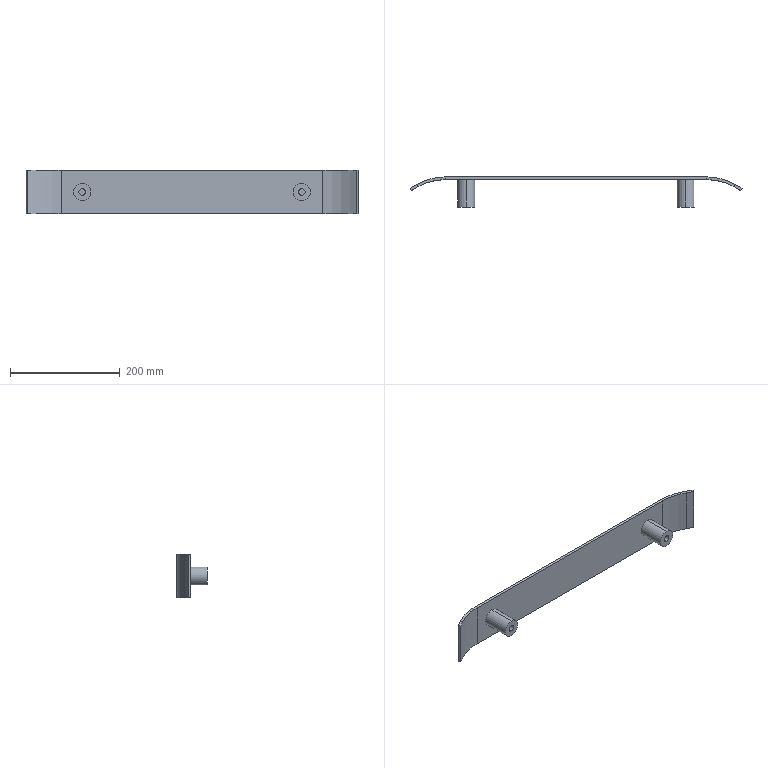Part | SolidWorks | features ICE 2, FlatPattern 1, SMBaseFlange 1, SheetMetal 1 | 1 solid | 34 faces | box 604.961 x 55 x 80 mm | volume 316837 mm3 | plane 22 | cylinder 12 | commonest cylinder face diameters 12 x4 32 x4 200 x2 210 x2
STEP:
#1=CARTESIAN_POINT('',(200.,-15.,6.));
#2=VERTEX_POINT('',#1);
#3=CARTESIAN_POINT('',(200.,-15.,-6.));
#4=VERTEX_POINT('',#3);
#5=CARTESIAN_POINT('',(200.,-15.,0.));
#6=DIRECTION('',(0.,-1.,0.));
#7=DIRECTION('',(0.,0.,-1.));
#8=AXIS2_PLACEMENT_3D('',#5,#6,#7);
#9=CIRCLE('',#8,6.);
#10=EDGE_CURVE('',#2,#4,#9,.T.);
#11=ORIENTED_EDGE('',*,*,#10,.F.);
#12=CARTESIAN_POINT('',(200.,-50.,6.));
#13=VERTEX_POINT('',#12);
#14=CARTESIAN_POINT('',(200.,-15.,6.));
#15=DIRECTION('',(0.,-1.,0.));
#16=VECTOR('',#15,1000.);
#17=LINE('',#14,#16);
#18=EDGE_CURVE('',#2,#13,#17,.T.);
#19=ORIENTED_EDGE('',*,*,#18,.T.);
#20=CARTESIAN_POINT('',(200.,-50.,-6.));
#21=VERTEX_POINT('',#20);
#22=CARTESIAN_POINT('',(200.,-50.,0.));
#23=DIRECTION('',(0.,-1.,0.));
#24=DIRECTION('',(0.,0.,-1.));
#25=AXIS2_PLACEMENT_3D('',#22,#23,#24);
#26=CIRCLE('',#25,6.);
#27=EDGE_CURVE('',#13,#21,#26,.T.);
#28=ORIENTED_EDGE('',*,*,#27,.T.);
#29=CARTESIAN_POINT('',(200.,-15.,-6.));
#30=DIRECTION('',(0.,-1.,0.));
#31=VECTOR('',#30,1000.);
#32=LINE('',#29,#31);
#33=EDGE_CURVE('',#4,#21,#32,.T.);
#34=ORIENTED_EDGE('',*,*,#33,.F.);
#35=EDGE_LOOP('',(#11,#19,#28,#34));
#36=FACE_OUTER_BOUND('',#35,.T.);
#37=CARTESIAN_POINT('',(200.,-15.,0.));
#38=DIRECTION('',(0.,-1.,0.));
#39=DIRECTION('',(0.,0.,-1.));
#40=AXIS2_PLACEMENT_3D('',#37,#38,#39);
#41=CYLINDRICAL_SURFACE('',#40,6.);
#42=ADVANCED_FACE('',(#36),#41,.F.);
#43=CARTESIAN_POINT('',(-200.,-15.,6.));
#44=VERTEX_POINT('',#43);
#45=CARTESIAN_POINT('',(-200.,-15.,-6.));
#46=VERTEX_POINT('',#45);
#47=CARTESIAN_POINT('',(-200.,-15.,0.));
#48=DIRECTION('',(0.,-1.,0.));
#49=DIRECTION('',(0.,0.,-1.));
#50=AXIS2_PLACEMENT_3D('',#47,#48,#49);
#51=CIRCLE('',#50,6.);
#52=EDGE_CURVE('',#44,#46,#51,.T.);
#53=ORIENTED_EDGE('',*,*,#52,.F.);
#54=CARTESIAN_POINT('',(-200.,-50.,6.));
#55=VERTEX_POINT('',#54);
#56=CARTESIAN_POINT('',(-200.,-15.,6.));
#57=DIRECTION('',(0.,-1.,0.));
#58=VECTOR('',#57,1000.);
#59=LINE('',#56,#58);
#60=EDGE_CURVE('',#44,#55,#59,.T.);
#61=ORIENTED_EDGE('',*,*,#60,.T.);
#62=CARTESIAN_POINT('',(-200.,-50.,-6.));
#63=VERTEX_POINT('',#62);
#64=CARTESIAN_POINT('',(-200.,-50.,0.));
#65=DIRECTION('',(0.,-1.,0.));
#66=DIRECTION('',(0.,0.,-1.));
#67=AXIS2_PLACEMENT_3D('',#64,#65,#66);
#68=CIRCLE('',#67,6.);
#69=EDGE_CURVE('',#55,#63,#68,.T.);
#70=ORIENTED_EDGE('',*,*,#69,.T.);
#71=CARTESIAN_POINT('',(-200.,-15.,-6.));
#72=DIRECTION('',(0.,-1.,0.));
#73=VECTOR('',#72,1000.);
#74=LINE('',#71,#73);
#75=EDGE_CURVE('',#46,#63,#74,.T.);
#76=ORIENTED_EDGE('',*,*,#75,.F.);
#77=EDGE_LOOP('',(#53,#61,#70,#76));
#78=FACE_OUTER_BOUND('',#77,.T.);
#79=CARTESIAN_POINT('',(-200.,-15.,0.));
#80=DIRECTION('',(0.,-1.,0.));
#81=DIRECTION('',(0.,0.,-1.));
#82=AXIS2_PLACEMENT_3D('',#79,#80,#81);
#83=CYLINDRICAL_SURFACE('',#82,6.);
#84=ADVANCED_FACE('',(#78),#83,.F.);
#85=CARTESIAN_POINT('',(-200.,-50.,-16.));
#86=VERTEX_POINT('',#85);
#87=CARTESIAN_POINT('',(-200.,-50.,16.));
#88=VERTEX_POINT('',#87);
#89=CARTESIAN_POINT('',(-200.,-50.,0.));
#90=DIRECTION('',(0.,-1.,0.));
#91=DIRECTION('',(0.,0.,-1.));
#92=AXIS2_PLACEMENT_3D('',#89,#90,#91);
#93=CIRCLE('',#92,16.);
#94=EDGE_CURVE('',#86,#88,#93,.T.);
#95=ORIENTED_EDGE('',*,*,#94,.F.);
#96=CARTESIAN_POINT('',(-200.,0.,-16.));
#97=VERTEX_POINT('',#96);
#98=CARTESIAN_POINT('',(-200.,-50.,-16.));
#99=DIRECTION('',(0.,1.,0.));
#100=VECTOR('',#99,1000.);
#101=LINE('',#98,#100);
#102=EDGE_CURVE('',#86,#97,#101,.T.);
#103=ORIENTED_EDGE('',*,*,#102,.T.);
#104=CARTESIAN_POINT('',(-200.,0.,16.));
#105=VERTEX_POINT('',#104);
#106=CARTESIAN_POINT('',(-200.,0.,0.));
#107=DIRECTION('',(0.,-1.,0.));
#108=DIRECTION('',(0.,0.,-1.));
#109=AXIS2_PLACEMENT_3D('',#106,#107,#108);
#110=CIRCLE('',#109,16.);
#111=EDGE_CURVE('',#97,#105,#110,.T.);
#112=ORIENTED_EDGE('',*,*,#111,.T.);
#113=CARTESIAN_POINT('',(-200.,-50.,16.));
#114=DIRECTION('',(0.,1.,0.));
#115=VECTOR('',#114,1000.);
#116=LINE('',#113,#115);
#117=EDGE_CURVE('',#88,#105,#116,.T.);
#118=ORIENTED_EDGE('',*,*,#117,.F.);
#119=EDGE_LOOP('',(#95,#103,#112,#118));
#120=FACE_OUTER_BOUND('',#119,.T.);
#121=CARTESIAN_POINT('',(-200.,-50.,0.));
#122=DIRECTION('',(0.,1.,0.));
#123=DIRECTION('',(0.,0.,1.));
#124=AXIS2_PLACEMENT_3D('',#121,#122,#123);
#125=CYLINDRICAL_SURFACE('',#124,16.);
#126=ADVANCED_FACE('',(#120),#125,.T.);
#127=CARTESIAN_POINT('',(200.,-50.,-16.));
#128=VERTEX_POINT('',#127);
#129=CARTESIAN_POINT('',(200.,-50.,16.));
#130=VERTEX_POINT('',#129);
#131=CARTESIAN_POINT('',(200.,-50.,0.));
#132=DIRECTION('',(0.,-1.,0.));
#133=DIRECTION('',(0.,0.,-1.));
#134=AXIS2_PLACEMENT_3D('',#131,#132,#133);
#135=CIRCLE('',#134,16.);
#136=EDGE_CURVE('',#128,#130,#135,.T.);
#137=ORIENTED_EDGE('',*,*,#136,.F.);
#138=CARTESIAN_POINT('',(200.,0.,-16.));
#139=VERTEX_POINT('',#138);
#140=CARTESIAN_POINT('',(200.,-50.,-16.));
#141=DIRECTION('',(0.,1.,0.));
#142=VECTOR('',#141,1000.);
#143=LINE('',#140,#142);
#144=EDGE_CURVE('',#128,#139,#143,.T.);
#145=ORIENTED_EDGE('',*,*,#144,.T.);
#146=CARTESIAN_POINT('',(200.,0.,16.));
#147=VERTEX_POINT('',#146);
#148=CARTESIAN_POINT('',(200.,0.,0.));
#149=DIRECTION('',(0.,-1.,0.));
#150=DIRECTION('',(0.,0.,-1.));
#151=AXIS2_PLACEMENT_3D('',#148,#149,#150);
#152=CIRCLE('',#151,16.);
#153=EDGE_CURVE('',#139,#147,#152,.T.);
#154=ORIENTED_EDGE('',*,*,#153,.T.);
#155=CARTESIAN_POINT('',(200.,-50.,16.));
#156=DIRECTION('',(0.,1.,0.));
#157=VECTOR('',#156,1000.);
#158=LINE('',#155,#157);
#159=EDGE_CURVE('',#130,#147,#158,.T.);
#160=ORIENTED_EDGE('',*,*,#159,.F.);
#161=EDGE_LOOP('',(#137,#145,#154,#160));
#162=FACE_OUTER_BOUND('',#161,.T.);
#163=CARTESIAN_POINT('',(200.,-50.,0.));
#164=DIRECTION('',(0.,1.,0.));
#165=DIRECTION('',(0.,0.,1.));
#166=AXIS2_PLACEMENT_3D('',#163,#164,#165);
#167=CYLINDRICAL_SURFACE('',#166,16.);
#168=ADVANCED_FACE('',(#162),#167,.T.);
#169=CARTESIAN_POINT('',(238.444,0.,40.));
#170=VERTEX_POINT('',#169);
#171=CARTESIAN_POINT('',(238.444,5.,40.));
#172=VERTEX_POINT('',#171);
#173=CARTESIAN_POINT('',(238.444,0.,40.));
#174=DIRECTION('',(0.,1.,0.));
#175=VECTOR('',#174,1000.);
#176=LINE('',#173,#175);
#177=EDGE_CURVE('',#170,#172,#176,.T.);
#178=ORIENTED_EDGE('',*,*,#177,.F.);
#179=CARTESIAN_POINT('',(288.057,-13.176,40.));
#180=VERTEX_POINT('',#179);
#181=CARTESIAN_POINT('',(238.444,-100.,40.));
#182=DIRECTION('',(0.,0.,1.));
#183=DIRECTION('',(-1.,0.,0.));
#184=AXIS2_PLACEMENT_3D('',#181,#182,#183);
#185=CIRCLE('',#184,100.);
#186=EDGE_CURVE('',#180,#170,#185,.T.);
#187=ORIENTED_EDGE('',*,*,#186,.F.);
#188=CARTESIAN_POINT('',(290.538,-8.834,40.));
#189=VERTEX_POINT('',#188);
#190=CARTESIAN_POINT('',(290.538,-8.834,40.));
#191=DIRECTION('',(-0.4961,-0.8682,0.));
#192=VECTOR('',#191,1000.);
#193=LINE('',#190,#192);
#194=EDGE_CURVE('',#189,#180,#193,.T.);
#195=ORIENTED_EDGE('',*,*,#194,.F.);
#196=CARTESIAN_POINT('',(238.444,-100.,40.));
#197=DIRECTION('',(0.,0.,1.));
#198=DIRECTION('',(1.,0.,0.));
#199=AXIS2_PLACEMENT_3D('',#196,#197,#198);
#200=CIRCLE('',#199,105.);
#201=EDGE_CURVE('',#189,#172,#200,.T.);
#202=ORIENTED_EDGE('',*,*,#201,.T.);
#203=EDGE_LOOP('',(#178,#187,#195,#202));
#204=FACE_OUTER_BOUND('',#203,.T.);
#205=CARTESIAN_POINT('',(238.444,0.,40.));
#206=DIRECTION('',(0.,0.,1.));
#207=DIRECTION('',(1.,0.,0.));
#208=AXIS2_PLACEMENT_3D('',#205,#206,#207);
#209=PLANE('',#208);
#210=ADVANCED_FACE('',(#204),#209,.T.);
#211=CARTESIAN_POINT('',(-238.444,0.,40.));
#212=VERTEX_POINT('',#211);
#213=CARTESIAN_POINT('',(-265.,0.,40.));
#214=DIRECTION('',(-1.,0.,0.));
#215=VECTOR('',#214,1000.);
#216=LINE('',#213,#215);
#217=EDGE_CURVE('',#170,#212,#216,.T.);
#218=ORIENTED_EDGE('',*,*,#217,.F.);
#219=ORIENTED_EDGE('',*,*,#177,.T.);
#220=CARTESIAN_POINT('',(-238.444,5.,40.));
#221=VERTEX_POINT('',#220);
#222=CARTESIAN_POINT('',(-265.,5.,40.));
#223=DIRECTION('',(-1.,0.,0.));
#224=VECTOR('',#223,1000.);
#225=LINE('',#222,#224);
#226=EDGE_CURVE('',#172,#221,#225,.T.);
#227=ORIENTED_EDGE('',*,*,#226,.T.);
#228=CARTESIAN_POINT('',(-238.444,5.,40.));
#229=DIRECTION('',(0.,-1.,0.));
#230=VECTOR('',#229,1000.);
#231=LINE('',#228,#230);
#232=EDGE_CURVE('',#221,#212,#231,.T.);
#233=ORIENTED_EDGE('',*,*,#232,.T.);
#234=EDGE_LOOP('',(#218,#219,#227,#233));
#235=FACE_OUTER_BOUND('',#234,.T.);
#236=CARTESIAN_POINT('',(290.538,-8.834,40.));
#237=DIRECTION('',(0.,0.,1.));
#238=DIRECTION('',(1.,0.,0.));
#239=AXIS2_PLACEMENT_3D('',#236,#237,#238);
#240=PLANE('',#239);
#241=ADVANCED_FACE('',(#235),#240,.T.);
#242=CARTESIAN_POINT('',(288.057,-13.176,-40.));
#243=VERTEX_POINT('',#242);
#244=CARTESIAN_POINT('',(290.538,-8.834,-40.));
#245=VERTEX_POINT('',#244);
#246=CARTESIAN_POINT('',(288.057,-13.176,-40.));
#247=DIRECTION('',(0.4961,0.8682,0.));
#248=VECTOR('',#247,1000.);
#249=LINE('',#246,#248);
#250=EDGE_CURVE('',#243,#245,#249,.T.);
#251=ORIENTED_EDGE('',*,*,#250,.F.);
#252=CARTESIAN_POINT('',(238.444,0.,-40.));
#253=VERTEX_POINT('',#252);
#254=CARTESIAN_POINT('',(238.444,-100.,-40.));
#255=DIRECTION('',(0.,0.,1.));
#256=DIRECTION('',(-1.,0.,0.));
#257=AXIS2_PLACEMENT_3D('',#254,#255,#256);
#258=CIRCLE('',#257,100.);
#259=EDGE_CURVE('',#243,#253,#258,.T.);
#260=ORIENTED_EDGE('',*,*,#259,.T.);
#261=CARTESIAN_POINT('',(238.444,5.,-40.));
#262=VERTEX_POINT('',#261);
#263=CARTESIAN_POINT('',(238.444,5.,-40.));
#264=DIRECTION('',(0.,-1.,0.));
#265=VECTOR('',#264,1000.);
#266=LINE('',#263,#265);
#267=EDGE_CURVE('',#262,#253,#266,.T.);
#268=ORIENTED_EDGE('',*,*,#267,.F.);
#269=CARTESIAN_POINT('',(238.444,-100.,-40.));
#270=DIRECTION('',(0.,0.,1.));
#271=DIRECTION('',(1.,0.,0.));
#272=AXIS2_PLACEMENT_3D('',#269,#270,#271);
#273=CIRCLE('',#272,105.);
#274=EDGE_CURVE('',#245,#262,#273,.T.);
#275=ORIENTED_EDGE('',*,*,#274,.F.);
#276=EDGE_LOOP('',(#251,#260,#268,#275));
#277=FACE_OUTER_BOUND('',#276,.T.);
#278=CARTESIAN_POINT('',(288.057,-13.176,-40.));
#279=DIRECTION('',(0.,0.,-1.));
#280=DIRECTION('',(-1.,0.,0.));
#281=AXIS2_PLACEMENT_3D('',#278,#279,#280);
#282=PLANE('',#281);
#283=ADVANCED_FACE('',(#277),#282,.T.);
#284=CARTESIAN_POINT('',(300.,-20.,-40.));
#285=VERTEX_POINT('',#284);
#286=CARTESIAN_POINT('',(265.,0.,-40.));
#287=DIRECTION('',(-0.8682,0.4961,0.));
#288=VECTOR('',#287,1000.);
#289=LINE('',#286,#288);
#290=EDGE_CURVE('',#285,#243,#289,.T.);
#291=ORIENTED_EDGE('',*,*,#290,.T.);
#292=ORIENTED_EDGE('',*,*,#250,.T.);
#293=CARTESIAN_POINT('',(302.481,-15.659,-40.));
#294=VERTEX_POINT('',#293);
#295=CARTESIAN_POINT('',(267.481,4.341,-40.));
#296=DIRECTION('',(-0.8682,0.4961,0.));
#297=VECTOR('',#296,1000.);
#298=LINE('',#295,#297);
#299=EDGE_CURVE('',#294,#245,#298,.T.);
#300=ORIENTED_EDGE('',*,*,#299,.F.);
#301=CARTESIAN_POINT('',(302.481,-15.659,-40.));
#302=DIRECTION('',(-0.4961,-0.8682,0.));
#303=VECTOR('',#302,1000.);
#304=LINE('',#301,#303);
#305=EDGE_CURVE('',#294,#285,#304,.T.);
#306=ORIENTED_EDGE('',*,*,#305,.T.);
#307=EDGE_LOOP('',(#291,#292,#300,#306));
#308=FACE_OUTER_BOUND('',#307,.T.);
#309=CARTESIAN_POINT('',(238.444,5.,-40.));
#310=DIRECTION('',(0.,0.,-1.));
#311=DIRECTION('',(-1.,0.,0.));
#312=AXIS2_PLACEMENT_3D('',#309,#310,#311);
#313=PLANE('',#312);
#314=ADVANCED_FACE('',(#308),#313,.T.);
#315=CARTESIAN_POINT('',(-288.057,-13.176,40.));
#316=VERTEX_POINT('',#315);
#317=CARTESIAN_POINT('',(-290.538,-8.834,40.));
#318=VERTEX_POINT('',#317);
#319=CARTESIAN_POINT('',(-288.057,-13.176,40.));
#320=DIRECTION('',(-0.4961,0.8682,0.));
#321=VECTOR('',#320,1000.);
#322=LINE('',#319,#321);
#323=EDGE_CURVE('',#316,#318,#322,.T.);
#324=ORIENTED_EDGE('',*,*,#323,.F.);
#325=CARTESIAN_POINT('',(-238.444,-100.,40.));
#326=DIRECTION('',(0.,0.,1.));
#327=DIRECTION('',(-1.,0.,0.));
#328=AXIS2_PLACEMENT_3D('',#325,#326,#327);
#329=CIRCLE('',#328,100.);
#330=EDGE_CURVE('',#212,#316,#329,.T.);
#331=ORIENTED_EDGE('',*,*,#330,.F.);
#332=ORIENTED_EDGE('',*,*,#232,.F.);
#333=CARTESIAN_POINT('',(-238.444,-100.,40.));
#334=DIRECTION('',(0.,0.,1.));
#335=DIRECTION('',(1.,0.,0.));
#336=AXIS2_PLACEMENT_3D('',#333,#334,#335);
#337=CIRCLE('',#336,105.);
#338=EDGE_CURVE('',#221,#318,#337,.T.);
#339=ORIENTED_EDGE('',*,*,#338,.T.);
#340=EDGE_LOOP('',(#324,#331,#332,#339));
#341=FACE_OUTER_BOUND('',#340,.T.);
#342=CARTESIAN_POINT('',(-288.057,-13.176,40.));
#343=DIRECTION('',(0.,0.,1.));
#344=DIRECTION('',(1.,0.,0.));
#345=AXIS2_PLACEMENT_3D('',#342,#343,#344);
#346=PLANE('',#345);
#347=ADVANCED_FACE('',(#341),#346,.T.);
#348=CARTESIAN_POINT('',(-300.,-20.,40.));
#349=VERTEX_POINT('',#348);
#350=CARTESIAN_POINT('',(-265.,0.,40.));
#351=DIRECTION('',(-0.8682,-0.4961,0.));
#352=VECTOR('',#351,1000.);
#353=LINE('',#350,#352);
#354=EDGE_CURVE('',#316,#349,#353,.T.);
#355=ORIENTED_EDGE('',*,*,#354,.F.);
#356=ORIENTED_EDGE('',*,*,#323,.T.);
#357=CARTESIAN_POINT('',(-302.481,-15.659,40.));
#358=VERTEX_POINT('',#357);
#359=CARTESIAN_POINT('',(-267.481,4.341,40.));
#360=DIRECTION('',(-0.8682,-0.4961,0.));
#361=VECTOR('',#360,1000.);
#362=LINE('',#359,#361);
#363=EDGE_CURVE('',#318,#358,#362,.T.);
#364=ORIENTED_EDGE('',*,*,#363,.T.);
#365=CARTESIAN_POINT('',(-300.,-20.,40.));
#366=DIRECTION('',(-0.4961,0.8682,0.));
#367=VECTOR('',#366,1000.);
#368=LINE('',#365,#367);
#369=EDGE_CURVE('',#349,#358,#368,.T.);
#370=ORIENTED_EDGE('',*,*,#369,.F.);
#371=EDGE_LOOP('',(#355,#356,#364,#370));
#372=FACE_OUTER_BOUND('',#371,.T.);
#373=CARTESIAN_POINT('',(-238.444,5.,40.));
#374=DIRECTION('',(0.,0.,1.));
#375=DIRECTION('',(1.,0.,0.));
#376=AXIS2_PLACEMENT_3D('',#373,#374,#375);
#377=PLANE('',#376);
#378=ADVANCED_FACE('',(#372),#377,.T.);
#379=CARTESIAN_POINT('',(-238.444,0.,-40.));
#380=VERTEX_POINT('',#379);
#381=CARTESIAN_POINT('',(-238.444,5.,-40.));
#382=VERTEX_POINT('',#381);
#383=CARTESIAN_POINT('',(-238.444,0.,-40.));
#384=DIRECTION('',(0.,1.,0.));
#385=VECTOR('',#384,1000.);
#386=LINE('',#383,#385);
#387=EDGE_CURVE('',#380,#382,#386,.T.);
#388=ORIENTED_EDGE('',*,*,#387,.F.);
#389=CARTESIAN_POINT('',(-288.057,-13.176,-40.));
#390=VERTEX_POINT('',#389);
#391=CARTESIAN_POINT('',(-238.444,-100.,-40.));
#392=DIRECTION('',(0.,0.,1.));
#393=DIRECTION('',(-1.,0.,0.));
#394=AXIS2_PLACEMENT_3D('',#391,#392,#393);
#395=CIRCLE('',#394,100.);
#396=EDGE_CURVE('',#380,#390,#395,.T.);
#397=ORIENTED_EDGE('',*,*,#396,.T.);
#398=CARTESIAN_POINT('',(-290.538,-8.834,-40.));
#399=VERTEX_POINT('',#398);
#400=CARTESIAN_POINT('',(-290.538,-8.834,-40.));
#401=DIRECTION('',(0.4961,-0.8682,0.));
#402=VECTOR('',#401,1000.);
#403=LINE('',#400,#402);
#404=EDGE_CURVE('',#399,#390,#403,.T.);
#405=ORIENTED_EDGE('',*,*,#404,.F.);
#406=CARTESIAN_POINT('',(-238.444,-100.,-40.));
#407=DIRECTION('',(0.,0.,1.));
#408=DIRECTION('',(1.,0.,0.));
#409=AXIS2_PLACEMENT_3D('',#406,#407,#408);
#410=CIRCLE('',#409,105.);
#411=EDGE_CURVE('',#382,#399,#410,.T.);
#412=ORIENTED_EDGE('',*,*,#411,.F.);
#413=EDGE_LOOP('',(#388,#397,#405,#412));
#414=FACE_OUTER_BOUND('',#413,.T.);
#415=CARTESIAN_POINT('',(-238.444,0.,-40.));
#416=DIRECTION('',(0.,0.,-1.));
#417=DIRECTION('',(-1.,0.,0.));
#418=AXIS2_PLACEMENT_3D('',#415,#416,#417);
#419=PLANE('',#418);
#420=ADVANCED_FACE('',(#414),#419,.T.);
#421=CARTESIAN_POINT('',(-265.,0.,-40.));
#422=DIRECTION('',(-1.,0.,0.));
#423=VECTOR('',#422,1000.);
#424=LINE('',#421,#423);
#425=EDGE_CURVE('',#253,#380,#424,.T.);
#426=ORIENTED_EDGE('',*,*,#425,.T.);
#427=ORIENTED_EDGE('',*,*,#387,.T.);
#428=CARTESIAN_POINT('',(-265.,5.,-40.));
#429=DIRECTION('',(-1.,0.,0.));
#430=VECTOR('',#429,1000.);
#431=LINE('',#428,#430);
#432=EDGE_CURVE('',#262,#382,#431,.T.);
#433=ORIENTED_EDGE('',*,*,#432,.F.);
#434=ORIENTED_EDGE('',*,*,#267,.T.);
#435=EDGE_LOOP('',(#426,#427,#433,#434));
#436=FACE_OUTER_BOUND('',#435,.T.);
#437=CARTESIAN_POINT('',(-290.538,-8.834,-40.));
#438=DIRECTION('',(0.,0.,-1.));
#439=DIRECTION('',(-1.,0.,0.));
#440=AXIS2_PLACEMENT_3D('',#437,#438,#439);
#441=PLANE('',#440);
#442=ADVANCED_FACE('',(#436),#441,.T.);
#443=CARTESIAN_POINT('',(-302.481,-15.659,-40.));
#444=VERTEX_POINT('',#443);
#445=CARTESIAN_POINT('',(-267.481,4.341,-40.));
#446=DIRECTION('',(-0.8682,-0.4961,0.));
#447=VECTOR('',#446,1000.);
#448=LINE('',#445,#447);
#449=EDGE_CURVE('',#399,#444,#448,.T.);
#450=ORIENTED_EDGE('',*,*,#449,.T.);
#451=CARTESIAN_POINT('',(-302.481,-15.659,40.));
#452=DIRECTION('',(0.,0.,-1.));
#453=VECTOR('',#452,1000.);
#454=LINE('',#451,#453);
#455=EDGE_CURVE('',#358,#444,#454,.T.);
#456=ORIENTED_EDGE('',*,*,#455,.F.);
#457=ORIENTED_EDGE('',*,*,#363,.F.);
#458=CARTESIAN_POINT('',(-290.538,-8.834,40.));
#459=DIRECTION('',(0.,0.,-1.));
#460=VECTOR('',#459,1000.);
#461=LINE('',#458,#460);
#462=EDGE_CURVE('',#318,#399,#461,.T.);
#463=ORIENTED_EDGE('',*,*,#462,.T.);
#464=EDGE_LOOP('',(#450,#456,#457,#463));
#465=FACE_OUTER_BOUND('',#464,.T.);
#466=CARTESIAN_POINT('',(-267.481,4.341,40.));
#467=DIRECTION('',(0.4961,-0.8682,0.));
#468=DIRECTION('',(0.8682,0.4961,0.));
#469=AXIS2_PLACEMENT_3D('',#466,#467,#468);
#470=PLANE('',#469);
#471=ADVANCED_FACE('',(#465),#470,.F.);
#472=CARTESIAN_POINT('',(-300.,-20.,-40.));
#473=VERTEX_POINT('',#472);
#474=CARTESIAN_POINT('',(-300.,-20.,-40.));
#475=DIRECTION('',(-0.4961,0.8682,0.));
#476=VECTOR('',#475,1000.);
#477=LINE('',#474,#476);
#478=EDGE_CURVE('',#473,#444,#477,.T.);
#479=ORIENTED_EDGE('',*,*,#478,.F.);
#480=CARTESIAN_POINT('',(-300.,-20.,40.));
#481=DIRECTION('',(0.,0.,-1.));
#482=VECTOR('',#481,1000.);
#483=LINE('',#480,#482);
#484=EDGE_CURVE('',#349,#473,#483,.T.);
#485=ORIENTED_EDGE('',*,*,#484,.F.);
#486=ORIENTED_EDGE('',*,*,#369,.T.);
#487=ORIENTED_EDGE('',*,*,#455,.T.);
#488=EDGE_LOOP('',(#479,#485,#486,#487));
#489=FACE_OUTER_BOUND('',#488,.T.);
#490=CARTESIAN_POINT('',(-300.,-20.,40.));
#491=DIRECTION('',(-0.8682,-0.4961,0.));
#492=DIRECTION('',(0.4961,-0.8682,0.));
#493=AXIS2_PLACEMENT_3D('',#490,#491,#492);
#494=PLANE('',#493);
#495=ADVANCED_FACE('',(#489),#494,.T.);
#496=CARTESIAN_POINT('',(-265.,0.,-40.));
#497=DIRECTION('',(-0.8682,-0.4961,0.));
#498=VECTOR('',#497,1000.);
#499=LINE('',#496,#498);
#500=EDGE_CURVE('',#390,#473,#499,.T.);
#501=ORIENTED_EDGE('',*,*,#500,.F.);
#502=CARTESIAN_POINT('',(-288.057,-13.176,40.));
#503=DIRECTION('',(0.,0.,-1.));
#504=VECTOR('',#503,1000.);
#505=LINE('',#502,#504);
#506=EDGE_CURVE('',#316,#390,#505,.T.);
#507=ORIENTED_EDGE('',*,*,#506,.F.);
#508=ORIENTED_EDGE('',*,*,#354,.T.);
#509=ORIENTED_EDGE('',*,*,#484,.T.);
#510=EDGE_LOOP('',(#501,#507,#508,#509));
#511=FACE_OUTER_BOUND('',#510,.T.);
#512=CARTESIAN_POINT('',(-265.,0.,40.));
#513=DIRECTION('',(0.4961,-0.8682,0.));
#514=DIRECTION('',(0.8682,0.4961,0.));
#515=AXIS2_PLACEMENT_3D('',#512,#513,#514);
#516=PLANE('',#515);
#517=ADVANCED_FACE('',(#511),#516,.T.);
#518=ORIENTED_EDGE('',*,*,#396,.F.);
#519=CARTESIAN_POINT('',(-238.444,0.,40.));
#520=DIRECTION('',(0.,0.,-1.));
#521=VECTOR('',#520,1000.);
#522=LINE('',#519,#521);
#523=EDGE_CURVE('',#212,#380,#522,.T.);
#524=ORIENTED_EDGE('',*,*,#523,.F.);
#525=ORIENTED_EDGE('',*,*,#330,.T.);
#526=ORIENTED_EDGE('',*,*,#506,.T.);
#527=EDGE_LOOP('',(#518,#524,#525,#526));
#528=FACE_OUTER_BOUND('',#527,.T.);
#529=CARTESIAN_POINT('',(-238.444,-100.,40.));
#530=DIRECTION('',(0.,0.,-1.));
#531=DIRECTION('',(-1.,0.,0.));
#532=AXIS2_PLACEMENT_3D('',#529,#530,#531);
#533=CYLINDRICAL_SURFACE('',#532,100.);
#534=ADVANCED_FACE('',(#528),#533,.F.);
#535=CARTESIAN_POINT('',(-200.,0.,0.));
#536=DIRECTION('',(0.,-1.,0.));
#537=DIRECTION('',(0.,0.,-1.));
#538=AXIS2_PLACEMENT_3D('',#535,#536,#537);
#539=CIRCLE('',#538,16.);
#540=EDGE_CURVE('',#105,#97,#539,.T.);
#541=ORIENTED_EDGE('',*,*,#540,.F.);
#542=ORIENTED_EDGE('',*,*,#111,.F.);
#543=EDGE_LOOP('',(#541,#542));
#544=FACE_BOUND('',#543,.T.);
#545=CARTESIAN_POINT('',(200.,0.,0.));
#546=DIRECTION('',(0.,-1.,0.));
#547=DIRECTION('',(0.,0.,-1.));
#548=AXIS2_PLACEMENT_3D('',#545,#546,#547);
#549=CIRCLE('',#548,16.);
#550=EDGE_CURVE('',#147,#139,#549,.T.);
#551=ORIENTED_EDGE('',*,*,#550,.F.);
#552=ORIENTED_EDGE('',*,*,#153,.F.);
#553=EDGE_LOOP('',(#551,#552));
#554=FACE_BOUND('',#553,.T.);
#555=ORIENTED_EDGE('',*,*,#425,.F.);
#556=CARTESIAN_POINT('',(238.444,0.,40.));
#557=DIRECTION('',(0.,0.,-1.));
#558=VECTOR('',#557,1000.);
#559=LINE('',#556,#558);
#560=EDGE_CURVE('',#170,#253,#559,.T.);
#561=ORIENTED_EDGE('',*,*,#560,.F.);
#562=ORIENTED_EDGE('',*,*,#217,.T.);
#563=ORIENTED_EDGE('',*,*,#523,.T.);
#564=EDGE_LOOP('',(#555,#561,#562,#563));
#565=FACE_OUTER_BOUND('',#564,.T.);
#566=CARTESIAN_POINT('',(-265.,0.,40.));
#567=DIRECTION('',(0.,-1.,0.));
#568=DIRECTION('',(0.,0.,-1.));
#569=AXIS2_PLACEMENT_3D('',#566,#567,#568);
#570=PLANE('',#569);
#571=ADVANCED_FACE('',(#544,#554,#565),#570,.T.);
#572=ORIENTED_EDGE('',*,*,#259,.F.);
#573=CARTESIAN_POINT('',(288.057,-13.176,40.));
#574=DIRECTION('',(0.,0.,-1.));
#575=VECTOR('',#574,1000.);
#576=LINE('',#573,#575);
#577=EDGE_CURVE('',#180,#243,#576,.T.);
#578=ORIENTED_EDGE('',*,*,#577,.F.);
#579=ORIENTED_EDGE('',*,*,#186,.T.);
#580=ORIENTED_EDGE('',*,*,#560,.T.);
#581=EDGE_LOOP('',(#572,#578,#579,#580));
#582=FACE_OUTER_BOUND('',#581,.T.);
#583=CARTESIAN_POINT('',(238.444,-100.,40.));
#584=DIRECTION('',(0.,0.,-1.));
#585=DIRECTION('',(-1.,0.,0.));
#586=AXIS2_PLACEMENT_3D('',#583,#584,#585);
#587=CYLINDRICAL_SURFACE('',#586,100.);
#588=ADVANCED_FACE('',(#582),#587,.F.);
#589=ORIENTED_EDGE('',*,*,#290,.F.);
#590=CARTESIAN_POINT('',(300.,-20.,40.));
#591=VERTEX_POINT('',#590);
#592=CARTESIAN_POINT('',(300.,-20.,40.));
#593=DIRECTION('',(0.,0.,-1.));
#594=VECTOR('',#593,1000.);
#595=LINE('',#592,#594);
#596=EDGE_CURVE('',#591,#285,#595,.T.);
#597=ORIENTED_EDGE('',*,*,#596,.F.);
#598=CARTESIAN_POINT('',(265.,0.,40.));
#599=DIRECTION('',(-0.8682,0.4961,0.));
#600=VECTOR('',#599,1000.);
#601=LINE('',#598,#600);
#602=EDGE_CURVE('',#591,#180,#601,.T.);
#603=ORIENTED_EDGE('',*,*,#602,.T.);
#604=ORIENTED_EDGE('',*,*,#577,.T.);
#605=EDGE_LOOP('',(#589,#597,#603,#604));
#606=FACE_OUTER_BOUND('',#605,.T.);
#607=CARTESIAN_POINT('',(265.,0.,40.));
#608=DIRECTION('',(-0.4961,-0.8682,0.));
#609=DIRECTION('',(0.8682,-0.4961,0.));
#610=AXIS2_PLACEMENT_3D('',#607,#608,#609);
#611=PLANE('',#610);
#612=ADVANCED_FACE('',(#606),#611,.T.);
#613=ORIENTED_EDGE('',*,*,#305,.F.);
#614=CARTESIAN_POINT('',(302.481,-15.659,40.));
#615=VERTEX_POINT('',#614);
#616=CARTESIAN_POINT('',(302.481,-15.659,40.));
#617=DIRECTION('',(0.,0.,-1.));
#618=VECTOR('',#617,1000.);
#619=LINE('',#616,#618);
#620=EDGE_CURVE('',#615,#294,#619,.T.);
#621=ORIENTED_EDGE('',*,*,#620,.F.);
#622=CARTESIAN_POINT('',(302.481,-15.659,40.));
#623=DIRECTION('',(-0.4961,-0.8682,0.));
#624=VECTOR('',#623,1000.);
#625=LINE('',#622,#624);
#626=EDGE_CURVE('',#615,#591,#625,.T.);
#627=ORIENTED_EDGE('',*,*,#626,.T.);
#628=ORIENTED_EDGE('',*,*,#596,.T.);
#629=EDGE_LOOP('',(#613,#621,#627,#628));
#630=FACE_OUTER_BOUND('',#629,.T.);
#631=CARTESIAN_POINT('',(302.481,-15.659,40.));
#632=DIRECTION('',(0.8682,-0.4961,0.));
#633=DIRECTION('',(0.4961,0.8682,0.));
#634=AXIS2_PLACEMENT_3D('',#631,#632,#633);
#635=PLANE('',#634);
#636=ADVANCED_FACE('',(#630),#635,.T.);
#637=ORIENTED_EDGE('',*,*,#299,.T.);
#638=CARTESIAN_POINT('',(290.538,-8.834,40.));
#639=DIRECTION('',(0.,0.,-1.));
#640=VECTOR('',#639,1000.);
#641=LINE('',#638,#640);
#642=EDGE_CURVE('',#189,#245,#641,.T.);
#643=ORIENTED_EDGE('',*,*,#642,.F.);
#644=CARTESIAN_POINT('',(267.481,4.341,40.));
#645=DIRECTION('',(-0.8682,0.4961,0.));
#646=VECTOR('',#645,1000.);
#647=LINE('',#644,#646);
#648=EDGE_CURVE('',#615,#189,#647,.T.);
#649=ORIENTED_EDGE('',*,*,#648,.F.);
#650=ORIENTED_EDGE('',*,*,#620,.T.);
#651=EDGE_LOOP('',(#637,#643,#649,#650));
#652=FACE_OUTER_BOUND('',#651,.T.);
#653=CARTESIAN_POINT('',(267.481,4.341,40.));
#654=DIRECTION('',(-0.4961,-0.8682,0.));
#655=DIRECTION('',(0.8682,-0.4961,0.));
#656=AXIS2_PLACEMENT_3D('',#653,#654,#655);
#657=PLANE('',#656);
#658=ADVANCED_FACE('',(#652),#657,.F.);
#659=ORIENTED_EDGE('',*,*,#274,.T.);
#660=CARTESIAN_POINT('',(238.444,5.,40.));
#661=DIRECTION('',(0.,0.,-1.));
#662=VECTOR('',#661,1000.);
#663=LINE('',#660,#662);
#664=EDGE_CURVE('',#172,#262,#663,.T.);
#665=ORIENTED_EDGE('',*,*,#664,.F.);
#666=ORIENTED_EDGE('',*,*,#201,.F.);
#667=ORIENTED_EDGE('',*,*,#642,.T.);
#668=EDGE_LOOP('',(#659,#665,#666,#667));
#669=FACE_OUTER_BOUND('',#668,.T.);
#670=CARTESIAN_POINT('',(238.444,-100.,40.));
#671=DIRECTION('',(0.,0.,-1.));
#672=DIRECTION('',(-1.,0.,0.));
#673=AXIS2_PLACEMENT_3D('',#670,#671,#672);
#674=CYLINDRICAL_SURFACE('',#673,105.);
#675=ADVANCED_FACE('',(#669),#674,.T.);
#676=ORIENTED_EDGE('',*,*,#432,.T.);
#677=CARTESIAN_POINT('',(-238.444,5.,40.));
#678=DIRECTION('',(0.,0.,-1.));
#679=VECTOR('',#678,1000.);
#680=LINE('',#677,#679);
#681=EDGE_CURVE('',#221,#382,#680,.T.);
#682=ORIENTED_EDGE('',*,*,#681,.F.);
#683=ORIENTED_EDGE('',*,*,#226,.F.);
#684=ORIENTED_EDGE('',*,*,#664,.T.);
#685=EDGE_LOOP('',(#676,#682,#683,#684));
#686=FACE_OUTER_BOUND('',#685,.T.);
#687=CARTESIAN_POINT('',(-265.,5.,40.));
#688=DIRECTION('',(0.,-1.,0.));
#689=DIRECTION('',(0.,0.,-1.));
#690=AXIS2_PLACEMENT_3D('',#687,#688,#689);
#691=PLANE('',#690);
#692=ADVANCED_FACE('',(#686),#691,.F.);
#693=ORIENTED_EDGE('',*,*,#411,.T.);
#694=ORIENTED_EDGE('',*,*,#462,.F.);
#695=ORIENTED_EDGE('',*,*,#338,.F.);
#696=ORIENTED_EDGE('',*,*,#681,.T.);
#697=EDGE_LOOP('',(#693,#694,#695,#696));
#698=FACE_OUTER_BOUND('',#697,.T.);
#699=CARTESIAN_POINT('',(-238.444,-100.,40.));
#700=DIRECTION('',(0.,0.,-1.));
#701=DIRECTION('',(-1.,0.,0.));
#702=AXIS2_PLACEMENT_3D('',#699,#700,#701);
#703=CYLINDRICAL_SURFACE('',#702,105.);
#704=ADVANCED_FACE('',(#698),#703,.T.);
#705=ORIENTED_EDGE('',*,*,#648,.T.);
#706=ORIENTED_EDGE('',*,*,#194,.T.);
#707=ORIENTED_EDGE('',*,*,#602,.F.);
#708=ORIENTED_EDGE('',*,*,#626,.F.);
#709=EDGE_LOOP('',(#705,#706,#707,#708));
#710=FACE_OUTER_BOUND('',#709,.T.);
#711=CARTESIAN_POINT('',(-238.444,-100.,40.));
#712=DIRECTION('',(0.,0.,-1.));
#713=DIRECTION('',(-1.,0.,0.));
#714=AXIS2_PLACEMENT_3D('',#711,#712,#713);
#715=PLANE('',#714);
#716=ADVANCED_FACE('',(#710),#715,.F.);
#717=ORIENTED_EDGE('',*,*,#449,.F.);
#718=ORIENTED_EDGE('',*,*,#404,.T.);
#719=ORIENTED_EDGE('',*,*,#500,.T.);
#720=ORIENTED_EDGE('',*,*,#478,.T.);
#721=EDGE_LOOP('',(#717,#718,#719,#720));
#722=FACE_OUTER_BOUND('',#721,.T.);
#723=CARTESIAN_POINT('',(-238.444,-100.,-40.));
#724=DIRECTION('',(0.,0.,-1.));
#725=DIRECTION('',(-1.,0.,0.));
#726=AXIS2_PLACEMENT_3D('',#723,#724,#725);
#727=PLANE('',#726);
#728=ADVANCED_FACE('',(#722),#727,.T.);
#729=ORIENTED_EDGE('',*,*,#144,.F.);
#730=CARTESIAN_POINT('',(200.,-50.,0.));
#731=DIRECTION('',(0.,-1.,0.));
#732=DIRECTION('',(0.,0.,-1.));
#733=AXIS2_PLACEMENT_3D('',#730,#731,#732);
#734=CIRCLE('',#733,16.);
#735=EDGE_CURVE('',#130,#128,#734,.T.);
#736=ORIENTED_EDGE('',*,*,#735,.F.);
#737=ORIENTED_EDGE('',*,*,#159,.T.);
#738=ORIENTED_EDGE('',*,*,#550,.T.);
#739=EDGE_LOOP('',(#729,#736,#737,#738));
#740=FACE_OUTER_BOUND('',#739,.T.);
#741=CARTESIAN_POINT('',(200.,-50.,0.));
#742=DIRECTION('',(0.,1.,0.));
#743=DIRECTION('',(0.,0.,1.));
#744=AXIS2_PLACEMENT_3D('',#741,#742,#743);
#745=CYLINDRICAL_SURFACE('',#744,16.);
#746=ADVANCED_FACE('',(#740),#745,.T.);
#747=CARTESIAN_POINT('',(200.,-50.,0.));
#748=DIRECTION('',(0.,-1.,0.));
#749=DIRECTION('',(0.,0.,-1.));
#750=AXIS2_PLACEMENT_3D('',#747,#748,#749);
#751=CIRCLE('',#750,6.);
#752=EDGE_CURVE('',#21,#13,#751,.T.);
#753=ORIENTED_EDGE('',*,*,#752,.F.);
#754=ORIENTED_EDGE('',*,*,#27,.F.);
#755=EDGE_LOOP('',(#753,#754));
#756=FACE_BOUND('',#755,.T.);
#757=ORIENTED_EDGE('',*,*,#735,.T.);
#758=ORIENTED_EDGE('',*,*,#136,.T.);
#759=EDGE_LOOP('',(#757,#758));
#760=FACE_OUTER_BOUND('',#759,.T.);
#761=CARTESIAN_POINT('',(200.,-50.,0.));
#762=DIRECTION('',(0.,-1.,0.));
#763=DIRECTION('',(0.,0.,-1.));
#764=AXIS2_PLACEMENT_3D('',#761,#762,#763);
#765=PLANE('',#764);
#766=ADVANCED_FACE('',(#756,#760),#765,.T.);
#767=ORIENTED_EDGE('',*,*,#102,.F.);
#768=CARTESIAN_POINT('',(-200.,-50.,0.));
#769=DIRECTION('',(0.,-1.,0.));
#770=DIRECTION('',(0.,0.,-1.));
#771=AXIS2_PLACEMENT_3D('',#768,#769,#770);
#772=CIRCLE('',#771,16.);
#773=EDGE_CURVE('',#88,#86,#772,.T.);
#774=ORIENTED_EDGE('',*,*,#773,.F.);
#775=ORIENTED_EDGE('',*,*,#117,.T.);
#776=ORIENTED_EDGE('',*,*,#540,.T.);
#777=EDGE_LOOP('',(#767,#774,#775,#776));
#778=FACE_OUTER_BOUND('',#777,.T.);
#779=CARTESIAN_POINT('',(-200.,-50.,0.));
#780=DIRECTION('',(0.,1.,0.));
#781=DIRECTION('',(0.,0.,1.));
#782=AXIS2_PLACEMENT_3D('',#779,#780,#781);
#783=CYLINDRICAL_SURFACE('',#782,16.);
#784=ADVANCED_FACE('',(#778),#783,.T.);
#785=CARTESIAN_POINT('',(-200.,-50.,0.));
#786=DIRECTION('',(0.,-1.,0.));
#787=DIRECTION('',(0.,0.,-1.));
#788=AXIS2_PLACEMENT_3D('',#785,#786,#787);
#789=CIRCLE('',#788,6.);
#790=EDGE_CURVE('',#63,#55,#789,.T.);
#791=ORIENTED_EDGE('',*,*,#790,.F.);
#792=ORIENTED_EDGE('',*,*,#69,.F.);
#793=EDGE_LOOP('',(#791,#792));
#794=FACE_BOUND('',#793,.T.);
#795=ORIENTED_EDGE('',*,*,#773,.T.);
#796=ORIENTED_EDGE('',*,*,#94,.T.);
#797=EDGE_LOOP('',(#795,#796));
#798=FACE_OUTER_BOUND('',#797,.T.);
#799=CARTESIAN_POINT('',(-200.,-50.,0.));
#800=DIRECTION('',(0.,-1.,0.));
#801=DIRECTION('',(0.,0.,-1.));
#802=AXIS2_PLACEMENT_3D('',#799,#800,#801);
#803=PLANE('',#802);
#804=ADVANCED_FACE('',(#794,#798),#803,.T.);
#805=ORIENTED_EDGE('',*,*,#60,.F.);
#806=CARTESIAN_POINT('',(-200.,-15.,0.));
#807=DIRECTION('',(0.,-1.,0.));
#808=DIRECTION('',(0.,0.,-1.));
#809=AXIS2_PLACEMENT_3D('',#806,#807,#808);
#810=CIRCLE('',#809,6.);
#811=EDGE_CURVE('',#46,#44,#810,.T.);
#812=ORIENTED_EDGE('',*,*,#811,.F.);
#813=ORIENTED_EDGE('',*,*,#75,.T.);
#814=ORIENTED_EDGE('',*,*,#790,.T.);
#815=EDGE_LOOP('',(#805,#812,#813,#814));
#816=FACE_OUTER_BOUND('',#815,.T.);
#817=CARTESIAN_POINT('',(-200.,-15.,0.));
#818=DIRECTION('',(0.,-1.,0.));
#819=DIRECTION('',(0.,0.,-1.));
#820=AXIS2_PLACEMENT_3D('',#817,#818,#819);
#821=CYLINDRICAL_SURFACE('',#820,6.);
#822=ADVANCED_FACE('',(#816),#821,.F.);
#823=ORIENTED_EDGE('',*,*,#811,.T.);
#824=ORIENTED_EDGE('',*,*,#52,.T.);
#825=EDGE_LOOP('',(#823,#824));
#826=FACE_OUTER_BOUND('',#825,.T.);
#827=CARTESIAN_POINT('',(-200.,-15.,0.));
#828=DIRECTION('',(0.,-1.,0.));
#829=DIRECTION('',(0.,0.,-1.));
#830=AXIS2_PLACEMENT_3D('',#827,#828,#829);
#831=PLANE('',#830);
#832=ADVANCED_FACE('',(#826),#831,.T.);
#833=ORIENTED_EDGE('',*,*,#18,.F.);
#834=CARTESIAN_POINT('',(200.,-15.,0.));
#835=DIRECTION('',(0.,-1.,0.));
#836=DIRECTION('',(0.,0.,-1.));
#837=AXIS2_PLACEMENT_3D('',#834,#835,#836);
#838=CIRCLE('',#837,6.);
#839=EDGE_CURVE('',#4,#2,#838,.T.);
#840=ORIENTED_EDGE('',*,*,#839,.F.);
#841=ORIENTED_EDGE('',*,*,#33,.T.);
#842=ORIENTED_EDGE('',*,*,#752,.T.);
#843=EDGE_LOOP('',(#833,#840,#841,#842));
#844=FACE_OUTER_BOUND('',#843,.T.);
#845=CARTESIAN_POINT('',(200.,-15.,0.));
#846=DIRECTION('',(0.,-1.,0.));
#847=DIRECTION('',(0.,0.,-1.));
#848=AXIS2_PLACEMENT_3D('',#845,#846,#847);
#849=CYLINDRICAL_SURFACE('',#848,6.);
#850=ADVANCED_FACE('',(#844),#849,.F.);
#851=ORIENTED_EDGE('',*,*,#839,.T.);
#852=ORIENTED_EDGE('',*,*,#10,.T.);
#853=EDGE_LOOP('',(#851,#852));
#854=FACE_OUTER_BOUND('',#853,.T.);
#855=CARTESIAN_POINT('',(200.,-15.,0.));
#856=DIRECTION('',(0.,-1.,0.));
#857=DIRECTION('',(0.,0.,-1.));
#858=AXIS2_PLACEMENT_3D('',#855,#856,#857);
#859=PLANE('',#858);
#860=ADVANCED_FACE('',(#854),#859,.T.);
#861=CLOSED_SHELL('',(#42,#84,#126,#168,#210,#241,#283,#314,#347,#378,#420,#442,#471,#495,#517,#534,#571,#588,#612,#636,#658,#675,#692,#704,#716,#728,#746,#766,#784,#804,#822,#832,#850,#860));
#862=MANIFOLD_SOLID_BREP('',#861);
#863=CARTESIAN_POINT('',(0.,0.,0.));
#864=DIRECTION('',(0.,0.,1.));
#865=DIRECTION('',(1.,0.,0.));
#866=AXIS2_PLACEMENT_3D('',#863,#864,#865);
#867=(LENGTH_UNIT()NAMED_UNIT(*)SI_UNIT(.MILLI.,.METRE.));
#868=UNCERTAINTY_MEASURE_WITH_UNIT(LENGTH_MEASURE(0.00001),#867,'','');
#869=(NAMED_UNIT(*)PLANE_ANGLE_UNIT()SI_UNIT($,.RADIAN.));
#870=(NAMED_UNIT(*)SI_UNIT($,.STERADIAN.)SOLID_ANGLE_UNIT());
#871=(GEOMETRIC_REPRESENTATION_CONTEXT(3)GLOBAL_UNCERTAINTY_ASSIGNED_CONTEXT((#868))GLOBAL_UNIT_ASSIGNED_CONTEXT((#867,#869,#870))REPRESENTATION_CONTEXT('',''));
#872=ADVANCED_BREP_SHAPE_REPRESENTATION('',(#862,#866),#871);